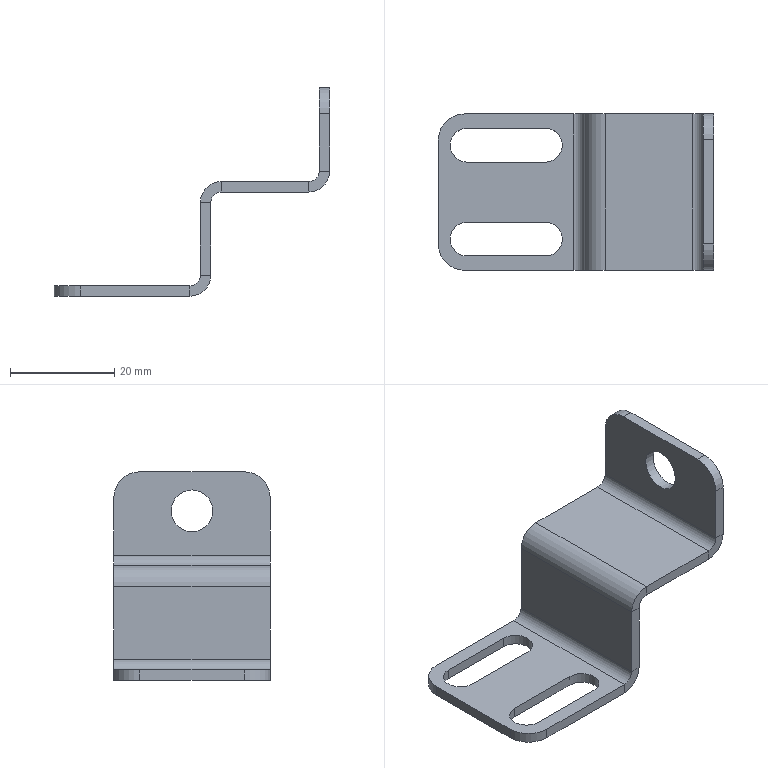Part | STEP file | JBJ-P-1006-10 | 1 solid | 43 faces | box 52.8 x 30 x 40 mm | volume 4550 mm3 | plane 28 | cylinder 15 | commonest cylinder face diameters 6.5 x4 8 x4 10 x4 4 x3
STEP:
#1=CARTESIAN_POINT('',(30.,30.,4.));
#2=VERTEX_POINT('',#1);
#3=CARTESIAN_POINT('',(28.,30.,4.));
#4=VERTEX_POINT('',#3);
#5=CARTESIAN_POINT('',(30.,30.,4.));
#6=DIRECTION('',(-1.,0.,0.));
#7=VECTOR('',#6,1000.);
#8=LINE('',#5,#7);
#9=EDGE_CURVE('',#2,#4,#8,.T.);
#10=ORIENTED_EDGE('',*,*,#9,.F.);
#11=CARTESIAN_POINT('',(26.,30.,0.));
#12=VERTEX_POINT('',#11);
#13=CARTESIAN_POINT('',(26.,30.,4.));
#14=DIRECTION('',(0.,-1.,0.));
#15=DIRECTION('',(0.,0.,1.));
#16=AXIS2_PLACEMENT_3D('',#13,#14,#15);
#17=CIRCLE('',#16,4.);
#18=EDGE_CURVE('',#12,#2,#17,.T.);
#19=ORIENTED_EDGE('',*,*,#18,.F.);
#20=CARTESIAN_POINT('',(26.,30.,2.));
#21=VERTEX_POINT('',#20);
#22=CARTESIAN_POINT('',(26.,30.,2.));
#23=DIRECTION('',(0.,0.,-1.));
#24=VECTOR('',#23,1000.);
#25=LINE('',#22,#24);
#26=EDGE_CURVE('',#21,#12,#25,.T.);
#27=ORIENTED_EDGE('',*,*,#26,.F.);
#28=CARTESIAN_POINT('',(26.,30.,4.));
#29=DIRECTION('',(0.,-1.,0.));
#30=DIRECTION('',(1.,0.,0.));
#31=AXIS2_PLACEMENT_3D('',#28,#29,#30);
#32=CIRCLE('',#31,2.);
#33=EDGE_CURVE('',#21,#4,#32,.T.);
#34=ORIENTED_EDGE('',*,*,#33,.T.);
#35=EDGE_LOOP('',(#10,#19,#27,#34));
#36=FACE_OUTER_BOUND('',#35,.T.);
#37=CARTESIAN_POINT('',(30.,30.,4.));
#38=DIRECTION('',(0.,1.,0.));
#39=DIRECTION('',(0.,0.,1.));
#40=AXIS2_PLACEMENT_3D('',#37,#38,#39);
#41=PLANE('',#40);
#42=ADVANCED_FACE('',(#36),#41,.T.);
#43=CARTESIAN_POINT('',(30.,30.,18.));
#44=VERTEX_POINT('',#43);
#45=CARTESIAN_POINT('',(30.,30.,0.));
#46=DIRECTION('',(0.,0.,1.));
#47=VECTOR('',#46,1000.);
#48=LINE('',#45,#47);
#49=EDGE_CURVE('',#2,#44,#48,.T.);
#50=ORIENTED_EDGE('',*,*,#49,.F.);
#51=ORIENTED_EDGE('',*,*,#9,.T.);
#52=CARTESIAN_POINT('',(28.,30.,18.));
#53=VERTEX_POINT('',#52);
#54=CARTESIAN_POINT('',(28.,30.,0.));
#55=DIRECTION('',(0.,0.,1.));
#56=VECTOR('',#55,1000.);
#57=LINE('',#54,#56);
#58=EDGE_CURVE('',#4,#53,#57,.T.);
#59=ORIENTED_EDGE('',*,*,#58,.T.);
#60=CARTESIAN_POINT('',(28.,30.,18.));
#61=DIRECTION('',(1.,0.,0.));
#62=VECTOR('',#61,1000.);
#63=LINE('',#60,#62);
#64=EDGE_CURVE('',#53,#44,#63,.T.);
#65=ORIENTED_EDGE('',*,*,#64,.T.);
#66=EDGE_LOOP('',(#50,#51,#59,#65));
#67=FACE_OUTER_BOUND('',#66,.T.);
#68=CARTESIAN_POINT('',(26.,30.,2.));
#69=DIRECTION('',(0.,1.,0.));
#70=DIRECTION('',(0.,0.,1.));
#71=AXIS2_PLACEMENT_3D('',#68,#69,#70);
#72=PLANE('',#71);
#73=ADVANCED_FACE('',(#67),#72,.T.);
#74=CARTESIAN_POINT('',(26.,0.,0.));
#75=VERTEX_POINT('',#74);
#76=CARTESIAN_POINT('',(26.,0.,2.));
#77=VERTEX_POINT('',#76);
#78=CARTESIAN_POINT('',(26.,0.,0.));
#79=DIRECTION('',(0.,0.,1.));
#80=VECTOR('',#79,1000.);
#81=LINE('',#78,#80);
#82=EDGE_CURVE('',#75,#77,#81,.T.);
#83=ORIENTED_EDGE('',*,*,#82,.F.);
#84=CARTESIAN_POINT('',(30.,0.,4.));
#85=VERTEX_POINT('',#84);
#86=CARTESIAN_POINT('',(26.,0.,4.));
#87=DIRECTION('',(0.,-1.,0.));
#88=DIRECTION('',(0.,0.,1.));
#89=AXIS2_PLACEMENT_3D('',#86,#87,#88);
#90=CIRCLE('',#89,4.);
#91=EDGE_CURVE('',#75,#85,#90,.T.);
#92=ORIENTED_EDGE('',*,*,#91,.T.);
#93=CARTESIAN_POINT('',(28.,0.,4.));
#94=VERTEX_POINT('',#93);
#95=CARTESIAN_POINT('',(28.,0.,4.));
#96=DIRECTION('',(1.,0.,0.));
#97=VECTOR('',#96,1000.);
#98=LINE('',#95,#97);
#99=EDGE_CURVE('',#94,#85,#98,.T.);
#100=ORIENTED_EDGE('',*,*,#99,.F.);
#101=CARTESIAN_POINT('',(26.,0.,4.));
#102=DIRECTION('',(0.,-1.,0.));
#103=DIRECTION('',(1.,0.,0.));
#104=AXIS2_PLACEMENT_3D('',#101,#102,#103);
#105=CIRCLE('',#104,2.);
#106=EDGE_CURVE('',#77,#94,#105,.T.);
#107=ORIENTED_EDGE('',*,*,#106,.F.);
#108=EDGE_LOOP('',(#83,#92,#100,#107));
#109=FACE_OUTER_BOUND('',#108,.T.);
#110=CARTESIAN_POINT('',(26.,0.,0.));
#111=DIRECTION('',(0.,-1.,0.));
#112=DIRECTION('',(0.,0.,-1.));
#113=AXIS2_PLACEMENT_3D('',#110,#111,#112);
#114=PLANE('',#113);
#115=ADVANCED_FACE('',(#109),#114,.T.);
#116=CARTESIAN_POINT('',(5.,0.,2.));
#117=VERTEX_POINT('',#116);
#118=CARTESIAN_POINT('',(0.,0.,2.));
#119=DIRECTION('',(1.,0.,0.));
#120=VECTOR('',#119,1000.);
#121=LINE('',#118,#120);
#122=EDGE_CURVE('',#117,#77,#121,.T.);
#123=ORIENTED_EDGE('',*,*,#122,.F.);
#124=CARTESIAN_POINT('',(5.,0.,0.));
#125=VERTEX_POINT('',#124);
#126=CARTESIAN_POINT('',(5.,0.,4.));
#127=DIRECTION('',(0.,0.,-1.));
#128=VECTOR('',#127,1000.);
#129=LINE('',#126,#128);
#130=EDGE_CURVE('',#117,#125,#129,.T.);
#131=ORIENTED_EDGE('',*,*,#130,.T.);
#132=CARTESIAN_POINT('',(0.,0.,0.));
#133=DIRECTION('',(1.,0.,0.));
#134=VECTOR('',#133,1000.);
#135=LINE('',#132,#134);
#136=EDGE_CURVE('',#125,#75,#135,.T.);
#137=ORIENTED_EDGE('',*,*,#136,.T.);
#138=ORIENTED_EDGE('',*,*,#82,.T.);
#139=EDGE_LOOP('',(#123,#131,#137,#138));
#140=FACE_OUTER_BOUND('',#139,.T.);
#141=CARTESIAN_POINT('',(28.,0.,4.));
#142=DIRECTION('',(0.,-1.,0.));
#143=DIRECTION('',(0.,0.,-1.));
#144=AXIS2_PLACEMENT_3D('',#141,#142,#143);
#145=PLANE('',#144);
#146=ADVANCED_FACE('',(#140),#145,.T.);
#147=CARTESIAN_POINT('',(32.,30.,20.));
#148=VERTEX_POINT('',#147);
#149=CARTESIAN_POINT('',(32.,30.,22.));
#150=VERTEX_POINT('',#149);
#151=CARTESIAN_POINT('',(32.,30.,20.));
#152=DIRECTION('',(0.,0.,1.));
#153=VECTOR('',#152,1000.);
#154=LINE('',#151,#153);
#155=EDGE_CURVE('',#148,#150,#154,.T.);
#156=ORIENTED_EDGE('',*,*,#155,.F.);
#157=CARTESIAN_POINT('',(32.,30.,18.));
#158=DIRECTION('',(0.,1.,0.));
#159=DIRECTION('',(0.,0.,-1.));
#160=AXIS2_PLACEMENT_3D('',#157,#158,#159);
#161=CIRCLE('',#160,2.);
#162=EDGE_CURVE('',#44,#148,#161,.T.);
#163=ORIENTED_EDGE('',*,*,#162,.F.);
#164=ORIENTED_EDGE('',*,*,#64,.F.);
#165=CARTESIAN_POINT('',(32.,30.,18.));
#166=DIRECTION('',(0.,1.,0.));
#167=DIRECTION('',(1.,0.,0.));
#168=AXIS2_PLACEMENT_3D('',#165,#166,#167);
#169=CIRCLE('',#168,4.);
#170=EDGE_CURVE('',#53,#150,#169,.T.);
#171=ORIENTED_EDGE('',*,*,#170,.T.);
#172=EDGE_LOOP('',(#156,#163,#164,#171));
#173=FACE_OUTER_BOUND('',#172,.T.);
#174=CARTESIAN_POINT('',(32.,30.,20.));
#175=DIRECTION('',(0.,1.,0.));
#176=DIRECTION('',(0.,0.,1.));
#177=AXIS2_PLACEMENT_3D('',#174,#175,#176);
#178=PLANE('',#177);
#179=ADVANCED_FACE('',(#173),#178,.T.);
#180=CARTESIAN_POINT('',(48.8,30.,20.));
#181=VERTEX_POINT('',#180);
#182=CARTESIAN_POINT('',(30.,30.,20.));
#183=DIRECTION('',(1.,0.,0.));
#184=VECTOR('',#183,1000.);
#185=LINE('',#182,#184);
#186=EDGE_CURVE('',#148,#181,#185,.T.);
#187=ORIENTED_EDGE('',*,*,#186,.F.);
#188=ORIENTED_EDGE('',*,*,#155,.T.);
#189=CARTESIAN_POINT('',(48.8,30.,22.));
#190=VERTEX_POINT('',#189);
#191=CARTESIAN_POINT('',(30.,30.,22.));
#192=DIRECTION('',(1.,0.,0.));
#193=VECTOR('',#192,1000.);
#194=LINE('',#191,#193);
#195=EDGE_CURVE('',#150,#190,#194,.T.);
#196=ORIENTED_EDGE('',*,*,#195,.T.);
#197=CARTESIAN_POINT('',(48.8,30.,22.));
#198=DIRECTION('',(0.,0.,-1.));
#199=VECTOR('',#198,1000.);
#200=LINE('',#197,#199);
#201=EDGE_CURVE('',#190,#181,#200,.T.);
#202=ORIENTED_EDGE('',*,*,#201,.T.);
#203=EDGE_LOOP('',(#187,#188,#196,#202));
#204=FACE_OUTER_BOUND('',#203,.T.);
#205=CARTESIAN_POINT('',(28.,30.,18.));
#206=DIRECTION('',(0.,1.,0.));
#207=DIRECTION('',(0.,0.,1.));
#208=AXIS2_PLACEMENT_3D('',#205,#206,#207);
#209=PLANE('',#208);
#210=ADVANCED_FACE('',(#204),#209,.T.);
#211=CARTESIAN_POINT('',(30.,0.,18.));
#212=VERTEX_POINT('',#211);
#213=CARTESIAN_POINT('',(28.,0.,18.));
#214=VERTEX_POINT('',#213);
#215=CARTESIAN_POINT('',(30.,0.,18.));
#216=DIRECTION('',(-1.,0.,0.));
#217=VECTOR('',#216,1000.);
#218=LINE('',#215,#217);
#219=EDGE_CURVE('',#212,#214,#218,.T.);
#220=ORIENTED_EDGE('',*,*,#219,.F.);
#221=CARTESIAN_POINT('',(32.,0.,20.));
#222=VERTEX_POINT('',#221);
#223=CARTESIAN_POINT('',(32.,0.,18.));
#224=DIRECTION('',(0.,1.,0.));
#225=DIRECTION('',(0.,0.,-1.));
#226=AXIS2_PLACEMENT_3D('',#223,#224,#225);
#227=CIRCLE('',#226,2.);
#228=EDGE_CURVE('',#212,#222,#227,.T.);
#229=ORIENTED_EDGE('',*,*,#228,.T.);
#230=CARTESIAN_POINT('',(32.,0.,22.));
#231=VERTEX_POINT('',#230);
#232=CARTESIAN_POINT('',(32.,0.,22.));
#233=DIRECTION('',(0.,0.,-1.));
#234=VECTOR('',#233,1000.);
#235=LINE('',#232,#234);
#236=EDGE_CURVE('',#231,#222,#235,.T.);
#237=ORIENTED_EDGE('',*,*,#236,.F.);
#238=CARTESIAN_POINT('',(32.,0.,18.));
#239=DIRECTION('',(0.,1.,0.));
#240=DIRECTION('',(1.,0.,0.));
#241=AXIS2_PLACEMENT_3D('',#238,#239,#240);
#242=CIRCLE('',#241,4.);
#243=EDGE_CURVE('',#214,#231,#242,.T.);
#244=ORIENTED_EDGE('',*,*,#243,.F.);
#245=EDGE_LOOP('',(#220,#229,#237,#244));
#246=FACE_OUTER_BOUND('',#245,.T.);
#247=CARTESIAN_POINT('',(30.,0.,18.));
#248=DIRECTION('',(0.,-1.,0.));
#249=DIRECTION('',(0.,0.,-1.));
#250=AXIS2_PLACEMENT_3D('',#247,#248,#249);
#251=PLANE('',#250);
#252=ADVANCED_FACE('',(#246),#251,.T.);
#253=CARTESIAN_POINT('',(30.,0.,0.));
#254=DIRECTION('',(0.,0.,1.));
#255=VECTOR('',#254,1000.);
#256=LINE('',#253,#255);
#257=EDGE_CURVE('',#85,#212,#256,.T.);
#258=ORIENTED_EDGE('',*,*,#257,.T.);
#259=ORIENTED_EDGE('',*,*,#219,.T.);
#260=CARTESIAN_POINT('',(28.,0.,0.));
#261=DIRECTION('',(0.,0.,1.));
#262=VECTOR('',#261,1000.);
#263=LINE('',#260,#262);
#264=EDGE_CURVE('',#94,#214,#263,.T.);
#265=ORIENTED_EDGE('',*,*,#264,.F.);
#266=ORIENTED_EDGE('',*,*,#99,.T.);
#267=EDGE_LOOP('',(#258,#259,#265,#266));
#268=FACE_OUTER_BOUND('',#267,.T.);
#269=CARTESIAN_POINT('',(32.,0.,22.));
#270=DIRECTION('',(0.,-1.,0.));
#271=DIRECTION('',(0.,0.,-1.));
#272=AXIS2_PLACEMENT_3D('',#269,#270,#271);
#273=PLANE('',#272);
#274=ADVANCED_FACE('',(#268),#273,.T.);
#275=CARTESIAN_POINT('',(52.8,30.,24.));
#276=VERTEX_POINT('',#275);
#277=CARTESIAN_POINT('',(50.8,30.,24.));
#278=VERTEX_POINT('',#277);
#279=CARTESIAN_POINT('',(52.8,30.,24.));
#280=DIRECTION('',(-1.,0.,0.));
#281=VECTOR('',#280,1000.);
#282=LINE('',#279,#281);
#283=EDGE_CURVE('',#276,#278,#282,.T.);
#284=ORIENTED_EDGE('',*,*,#283,.F.);
#285=CARTESIAN_POINT('',(48.8,30.,24.));
#286=DIRECTION('',(0.,-1.,0.));
#287=DIRECTION('',(0.,0.,1.));
#288=AXIS2_PLACEMENT_3D('',#285,#286,#287);
#289=CIRCLE('',#288,4.);
#290=EDGE_CURVE('',#181,#276,#289,.T.);
#291=ORIENTED_EDGE('',*,*,#290,.F.);
#292=ORIENTED_EDGE('',*,*,#201,.F.);
#293=CARTESIAN_POINT('',(48.8,30.,24.));
#294=DIRECTION('',(0.,-1.,0.));
#295=DIRECTION('',(1.,0.,0.));
#296=AXIS2_PLACEMENT_3D('',#293,#294,#295);
#297=CIRCLE('',#296,2.);
#298=EDGE_CURVE('',#190,#278,#297,.T.);
#299=ORIENTED_EDGE('',*,*,#298,.T.);
#300=EDGE_LOOP('',(#284,#291,#292,#299));
#301=FACE_OUTER_BOUND('',#300,.T.);
#302=CARTESIAN_POINT('',(52.8,30.,24.));
#303=DIRECTION('',(0.,1.,0.));
#304=DIRECTION('',(0.,0.,1.));
#305=AXIS2_PLACEMENT_3D('',#302,#303,#304);
#306=PLANE('',#305);
#307=ADVANCED_FACE('',(#301),#306,.T.);
#308=CARTESIAN_POINT('',(50.8,30.,35.));
#309=VERTEX_POINT('',#308);
#310=CARTESIAN_POINT('',(50.8,30.,20.));
#311=DIRECTION('',(0.,0.,1.));
#312=VECTOR('',#311,1000.);
#313=LINE('',#310,#312);
#314=EDGE_CURVE('',#278,#309,#313,.T.);
#315=ORIENTED_EDGE('',*,*,#314,.T.);
#316=CARTESIAN_POINT('',(52.8,30.,35.));
#317=VERTEX_POINT('',#316);
#318=CARTESIAN_POINT('',(48.8,30.,35.));
#319=DIRECTION('',(1.,0.,0.));
#320=VECTOR('',#319,1000.);
#321=LINE('',#318,#320);
#322=EDGE_CURVE('',#309,#317,#321,.T.);
#323=ORIENTED_EDGE('',*,*,#322,.T.);
#324=CARTESIAN_POINT('',(52.8,30.,20.));
#325=DIRECTION('',(0.,0.,1.));
#326=VECTOR('',#325,1000.);
#327=LINE('',#324,#326);
#328=EDGE_CURVE('',#276,#317,#327,.T.);
#329=ORIENTED_EDGE('',*,*,#328,.F.);
#330=ORIENTED_EDGE('',*,*,#283,.T.);
#331=EDGE_LOOP('',(#315,#323,#329,#330));
#332=FACE_OUTER_BOUND('',#331,.T.);
#333=CARTESIAN_POINT('',(48.8,30.,22.));
#334=DIRECTION('',(0.,1.,0.));
#335=DIRECTION('',(0.,0.,1.));
#336=AXIS2_PLACEMENT_3D('',#333,#334,#335);
#337=PLANE('',#336);
#338=ADVANCED_FACE('',(#332),#337,.T.);
#339=CARTESIAN_POINT('',(48.8,0.,20.));
#340=VERTEX_POINT('',#339);
#341=CARTESIAN_POINT('',(48.8,0.,22.));
#342=VERTEX_POINT('',#341);
#343=CARTESIAN_POINT('',(48.8,0.,20.));
#344=DIRECTION('',(0.,0.,1.));
#345=VECTOR('',#344,1000.);
#346=LINE('',#343,#345);
#347=EDGE_CURVE('',#340,#342,#346,.T.);
#348=ORIENTED_EDGE('',*,*,#347,.F.);
#349=CARTESIAN_POINT('',(52.8,0.,24.));
#350=VERTEX_POINT('',#349);
#351=CARTESIAN_POINT('',(48.8,0.,24.));
#352=DIRECTION('',(0.,-1.,0.));
#353=DIRECTION('',(0.,0.,1.));
#354=AXIS2_PLACEMENT_3D('',#351,#352,#353);
#355=CIRCLE('',#354,4.);
#356=EDGE_CURVE('',#340,#350,#355,.T.);
#357=ORIENTED_EDGE('',*,*,#356,.T.);
#358=CARTESIAN_POINT('',(50.8,0.,24.));
#359=VERTEX_POINT('',#358);
#360=CARTESIAN_POINT('',(50.8,0.,24.));
#361=DIRECTION('',(1.,0.,0.));
#362=VECTOR('',#361,1000.);
#363=LINE('',#360,#362);
#364=EDGE_CURVE('',#359,#350,#363,.T.);
#365=ORIENTED_EDGE('',*,*,#364,.F.);
#366=CARTESIAN_POINT('',(48.8,0.,24.));
#367=DIRECTION('',(0.,-1.,0.));
#368=DIRECTION('',(1.,0.,0.));
#369=AXIS2_PLACEMENT_3D('',#366,#367,#368);
#370=CIRCLE('',#369,2.);
#371=EDGE_CURVE('',#342,#359,#370,.T.);
#372=ORIENTED_EDGE('',*,*,#371,.F.);
#373=EDGE_LOOP('',(#348,#357,#365,#372));
#374=FACE_OUTER_BOUND('',#373,.T.);
#375=CARTESIAN_POINT('',(48.8,0.,20.));
#376=DIRECTION('',(0.,-1.,0.));
#377=DIRECTION('',(0.,0.,-1.));
#378=AXIS2_PLACEMENT_3D('',#375,#376,#377);
#379=PLANE('',#378);
#380=ADVANCED_FACE('',(#374),#379,.T.);
#381=CARTESIAN_POINT('',(30.,0.,20.));
#382=DIRECTION('',(1.,0.,0.));
#383=VECTOR('',#382,1000.);
#384=LINE('',#381,#383);
#385=EDGE_CURVE('',#222,#340,#384,.T.);
#386=ORIENTED_EDGE('',*,*,#385,.T.);
#387=ORIENTED_EDGE('',*,*,#347,.T.);
#388=CARTESIAN_POINT('',(30.,0.,22.));
#389=DIRECTION('',(1.,0.,0.));
#390=VECTOR('',#389,1000.);
#391=LINE('',#388,#390);
#392=EDGE_CURVE('',#231,#342,#391,.T.);
#393=ORIENTED_EDGE('',*,*,#392,.F.);
#394=ORIENTED_EDGE('',*,*,#236,.T.);
#395=EDGE_LOOP('',(#386,#387,#393,#394));
#396=FACE_OUTER_BOUND('',#395,.T.);
#397=CARTESIAN_POINT('',(50.8,0.,24.));
#398=DIRECTION('',(0.,-1.,0.));
#399=DIRECTION('',(0.,0.,-1.));
#400=AXIS2_PLACEMENT_3D('',#397,#398,#399);
#401=PLANE('',#400);
#402=ADVANCED_FACE('',(#396),#401,.T.);
#403=CARTESIAN_POINT('',(50.8,15.,36.5));
#404=VERTEX_POINT('',#403);
#405=CARTESIAN_POINT('',(50.8,15.,32.5));
#406=DIRECTION('',(-1.,0.,0.));
#407=DIRECTION('',(0.,0.,1.));
#408=AXIS2_PLACEMENT_3D('',#405,#406,#407);
#409=CIRCLE('',#408,4.);
#410=EDGE_CURVE('',#404,#404,#409,.T.);
#411=ORIENTED_EDGE('',*,*,#410,.F.);
#412=EDGE_LOOP('',(#411));
#413=FACE_BOUND('',#412,.T.);
#414=CARTESIAN_POINT('',(50.8,0.,35.));
#415=VERTEX_POINT('',#414);
#416=CARTESIAN_POINT('',(50.8,0.,20.));
#417=DIRECTION('',(0.,0.,1.));
#418=VECTOR('',#417,1000.);
#419=LINE('',#416,#418);
#420=EDGE_CURVE('',#359,#415,#419,.T.);
#421=ORIENTED_EDGE('',*,*,#420,.T.);
#422=CARTESIAN_POINT('',(50.8,5.,40.));
#423=VERTEX_POINT('',#422);
#424=CARTESIAN_POINT('',(50.8,5.,35.));
#425=DIRECTION('',(-1.,0.,0.));
#426=DIRECTION('',(0.,0.,-1.));
#427=AXIS2_PLACEMENT_3D('',#424,#425,#426);
#428=CIRCLE('',#427,5.);
#429=EDGE_CURVE('',#415,#423,#428,.T.);
#430=ORIENTED_EDGE('',*,*,#429,.T.);
#431=CARTESIAN_POINT('',(50.8,25.,40.));
#432=VERTEX_POINT('',#431);
#433=CARTESIAN_POINT('',(50.8,30.,40.));
#434=DIRECTION('',(0.,-1.,0.));
#435=VECTOR('',#434,1000.);
#436=LINE('',#433,#435);
#437=EDGE_CURVE('',#432,#423,#436,.T.);
#438=ORIENTED_EDGE('',*,*,#437,.F.);
#439=CARTESIAN_POINT('',(50.8,25.,35.));
#440=DIRECTION('',(-1.,0.,0.));
#441=DIRECTION('',(0.,0.,-1.));
#442=AXIS2_PLACEMENT_3D('',#439,#440,#441);
#443=CIRCLE('',#442,5.);
#444=EDGE_CURVE('',#432,#309,#443,.T.);
#445=ORIENTED_EDGE('',*,*,#444,.T.);
#446=ORIENTED_EDGE('',*,*,#314,.F.);
#447=CARTESIAN_POINT('',(50.8,30.,24.));
#448=DIRECTION('',(0.,-1.,0.));
#449=VECTOR('',#448,1000.);
#450=LINE('',#447,#449);
#451=EDGE_CURVE('',#278,#359,#450,.T.);
#452=ORIENTED_EDGE('',*,*,#451,.T.);
#453=EDGE_LOOP('',(#421,#430,#438,#445,#446,#452));
#454=FACE_OUTER_BOUND('',#453,.T.);
#455=CARTESIAN_POINT('',(50.8,30.,20.));
#456=DIRECTION('',(1.,0.,0.));
#457=DIRECTION('',(0.,0.,-1.));
#458=AXIS2_PLACEMENT_3D('',#455,#456,#457);
#459=PLANE('',#458);
#460=ADVANCED_FACE('',(#413,#454),#459,.F.);
#461=ORIENTED_EDGE('',*,*,#437,.T.);
#462=CARTESIAN_POINT('',(52.8,5.,40.));
#463=VERTEX_POINT('',#462);
#464=CARTESIAN_POINT('',(52.8,5.,40.));
#465=DIRECTION('',(1.,0.,0.));
#466=VECTOR('',#465,1000.);
#467=LINE('',#464,#466);
#468=EDGE_CURVE('',#423,#463,#467,.T.);
#469=ORIENTED_EDGE('',*,*,#468,.T.);
#470=CARTESIAN_POINT('',(52.8,25.,40.));
#471=VERTEX_POINT('',#470);
#472=CARTESIAN_POINT('',(52.8,30.,40.));
#473=DIRECTION('',(0.,-1.,0.));
#474=VECTOR('',#473,1000.);
#475=LINE('',#472,#474);
#476=EDGE_CURVE('',#471,#463,#475,.T.);
#477=ORIENTED_EDGE('',*,*,#476,.F.);
#478=CARTESIAN_POINT('',(52.8,25.,40.));
#479=DIRECTION('',(-1.,0.,0.));
#480=VECTOR('',#479,1000.);
#481=LINE('',#478,#480);
#482=EDGE_CURVE('',#471,#432,#481,.T.);
#483=ORIENTED_EDGE('',*,*,#482,.T.);
#484=EDGE_LOOP('',(#461,#469,#477,#483));
#485=FACE_OUTER_BOUND('',#484,.T.);
#486=CARTESIAN_POINT('',(52.8,30.,40.));
#487=DIRECTION('',(0.,0.,1.));
#488=DIRECTION('',(1.,0.,0.));
#489=AXIS2_PLACEMENT_3D('',#486,#487,#488);
#490=PLANE('',#489);
#491=ADVANCED_FACE('',(#485),#490,.T.);
#492=CARTESIAN_POINT('',(52.8,15.,28.5));
#493=VERTEX_POINT('',#492);
#494=CARTESIAN_POINT('',(52.8,15.,32.5));
#495=DIRECTION('',(1.,0.,0.));
#496=DIRECTION('',(0.,0.,-1.));
#497=AXIS2_PLACEMENT_3D('',#494,#495,#496);
#498=CIRCLE('',#497,4.);
#499=EDGE_CURVE('',#493,#493,#498,.T.);
#500=ORIENTED_EDGE('',*,*,#499,.F.);
#501=EDGE_LOOP('',(#500));
#502=FACE_BOUND('',#501,.T.);
#503=ORIENTED_EDGE('',*,*,#476,.T.);
#504=CARTESIAN_POINT('',(52.8,0.,35.));
#505=VERTEX_POINT('',#504);
#506=CARTESIAN_POINT('',(52.8,5.,35.));
#507=DIRECTION('',(1.,0.,0.));
#508=DIRECTION('',(0.,0.,-1.));
#509=AXIS2_PLACEMENT_3D('',#506,#507,#508);
#510=CIRCLE('',#509,5.);
#511=EDGE_CURVE('',#463,#505,#510,.T.);
#512=ORIENTED_EDGE('',*,*,#511,.T.);
#513=CARTESIAN_POINT('',(52.8,0.,20.));
#514=DIRECTION('',(0.,0.,1.));
#515=VECTOR('',#514,1000.);
#516=LINE('',#513,#515);
#517=EDGE_CURVE('',#350,#505,#516,.T.);
#518=ORIENTED_EDGE('',*,*,#517,.F.);
#519=CARTESIAN_POINT('',(52.8,30.,24.));
#520=DIRECTION('',(0.,-1.,0.));
#521=VECTOR('',#520,1000.);
#522=LINE('',#519,#521);
#523=EDGE_CURVE('',#276,#350,#522,.T.);
#524=ORIENTED_EDGE('',*,*,#523,.F.);
#525=ORIENTED_EDGE('',*,*,#328,.T.);
#526=CARTESIAN_POINT('',(52.8,25.,35.));
#527=DIRECTION('',(1.,0.,0.));
#528=DIRECTION('',(0.,0.,-1.));
#529=AXIS2_PLACEMENT_3D('',#526,#527,#528);
#530=CIRCLE('',#529,5.);
#531=EDGE_CURVE('',#317,#471,#530,.T.);
#532=ORIENTED_EDGE('',*,*,#531,.T.);
#533=EDGE_LOOP('',(#503,#512,#518,#524,#525,#532));
#534=FACE_OUTER_BOUND('',#533,.T.);
#535=CARTESIAN_POINT('',(52.8,30.,20.));
#536=DIRECTION('',(1.,0.,0.));
#537=DIRECTION('',(0.,0.,-1.));
#538=AXIS2_PLACEMENT_3D('',#535,#536,#537);
#539=PLANE('',#538);
#540=ADVANCED_FACE('',(#502,#534),#539,.T.);
#541=ORIENTED_EDGE('',*,*,#356,.F.);
#542=CARTESIAN_POINT('',(48.8,30.,20.));
#543=DIRECTION('',(0.,-1.,0.));
#544=VECTOR('',#543,1000.);
#545=LINE('',#542,#544);
#546=EDGE_CURVE('',#181,#340,#545,.T.);
#547=ORIENTED_EDGE('',*,*,#546,.F.);
#548=ORIENTED_EDGE('',*,*,#290,.T.);
#549=ORIENTED_EDGE('',*,*,#523,.T.);
#550=EDGE_LOOP('',(#541,#547,#548,#549));
#551=FACE_OUTER_BOUND('',#550,.T.);
#552=CARTESIAN_POINT('',(48.8,30.,24.));
#553=DIRECTION('',(0.,-1.,0.));
#554=DIRECTION('',(0.,0.,-1.));
#555=AXIS2_PLACEMENT_3D('',#552,#553,#554);
#556=CYLINDRICAL_SURFACE('',#555,4.);
#557=ADVANCED_FACE('',(#551),#556,.T.);
#558=ORIENTED_EDGE('',*,*,#385,.F.);
#559=CARTESIAN_POINT('',(32.,30.,20.));
#560=DIRECTION('',(0.,-1.,0.));
#561=VECTOR('',#560,1000.);
#562=LINE('',#559,#561);
#563=EDGE_CURVE('',#148,#222,#562,.T.);
#564=ORIENTED_EDGE('',*,*,#563,.F.);
#565=ORIENTED_EDGE('',*,*,#186,.T.);
#566=ORIENTED_EDGE('',*,*,#546,.T.);
#567=EDGE_LOOP('',(#558,#564,#565,#566));
#568=FACE_OUTER_BOUND('',#567,.T.);
#569=CARTESIAN_POINT('',(30.,30.,20.));
#570=DIRECTION('',(0.,0.,-1.));
#571=DIRECTION('',(-1.,0.,0.));
#572=AXIS2_PLACEMENT_3D('',#569,#570,#571);
#573=PLANE('',#572);
#574=ADVANCED_FACE('',(#568),#573,.T.);
#575=ORIENTED_EDGE('',*,*,#228,.F.);
#576=CARTESIAN_POINT('',(30.,30.,18.));
#577=DIRECTION('',(0.,-1.,0.));
#578=VECTOR('',#577,1000.);
#579=LINE('',#576,#578);
#580=EDGE_CURVE('',#44,#212,#579,.T.);
#581=ORIENTED_EDGE('',*,*,#580,.F.);
#582=ORIENTED_EDGE('',*,*,#162,.T.);
#583=ORIENTED_EDGE('',*,*,#563,.T.);
#584=EDGE_LOOP('',(#575,#581,#582,#583));
#585=FACE_OUTER_BOUND('',#584,.T.);
#586=CARTESIAN_POINT('',(32.,30.,18.));
#587=DIRECTION('',(0.,-1.,0.));
#588=DIRECTION('',(0.,0.,-1.));
#589=AXIS2_PLACEMENT_3D('',#586,#587,#588);
#590=CYLINDRICAL_SURFACE('',#589,2.);
#591=ADVANCED_FACE('',(#585),#590,.F.);
#592=ORIENTED_EDGE('',*,*,#257,.F.);
#593=CARTESIAN_POINT('',(30.,30.,4.));
#594=DIRECTION('',(0.,-1.,0.));
#595=VECTOR('',#594,1000.);
#596=LINE('',#593,#595);
#597=EDGE_CURVE('',#2,#85,#596,.T.);
#598=ORIENTED_EDGE('',*,*,#597,.F.);
#599=ORIENTED_EDGE('',*,*,#49,.T.);
#600=ORIENTED_EDGE('',*,*,#580,.T.);
#601=EDGE_LOOP('',(#592,#598,#599,#600));
#602=FACE_OUTER_BOUND('',#601,.T.);
#603=CARTESIAN_POINT('',(30.,30.,0.));
#604=DIRECTION('',(1.,0.,0.));
#605=DIRECTION('',(0.,0.,-1.));
#606=AXIS2_PLACEMENT_3D('',#603,#604,#605);
#607=PLANE('',#606);
#608=ADVANCED_FACE('',(#602),#607,.T.);
#609=ORIENTED_EDGE('',*,*,#91,.F.);
#610=CARTESIAN_POINT('',(26.,30.,0.));
#611=DIRECTION('',(0.,-1.,0.));
#612=VECTOR('',#611,1000.);
#613=LINE('',#610,#612);
#614=EDGE_CURVE('',#12,#75,#613,.T.);
#615=ORIENTED_EDGE('',*,*,#614,.F.);
#616=ORIENTED_EDGE('',*,*,#18,.T.);
#617=ORIENTED_EDGE('',*,*,#597,.T.);
#618=EDGE_LOOP('',(#609,#615,#616,#617));
#619=FACE_OUTER_BOUND('',#618,.T.);
#620=CARTESIAN_POINT('',(26.,30.,4.));
#621=DIRECTION('',(0.,-1.,0.));
#622=DIRECTION('',(0.,0.,-1.));
#623=AXIS2_PLACEMENT_3D('',#620,#621,#622);
#624=CYLINDRICAL_SURFACE('',#623,4.);
#625=ADVANCED_FACE('',(#619),#624,.T.);
#626=CARTESIAN_POINT('',(20.5,27.25,0.));
#627=VERTEX_POINT('',#626);
#628=CARTESIAN_POINT('',(20.5,20.75,0.));
#629=VERTEX_POINT('',#628);
#630=CARTESIAN_POINT('',(20.5,24.,0.));
#631=DIRECTION('',(0.,0.,-1.));
#632=DIRECTION('',(-1.,0.,0.));
#633=AXIS2_PLACEMENT_3D('',#630,#631,#632);
#634=CIRCLE('',#633,3.25);
#635=EDGE_CURVE('',#627,#629,#634,.T.);
#636=ORIENTED_EDGE('',*,*,#635,.F.);
#637=CARTESIAN_POINT('',(5.5,27.25,0.));
#638=VERTEX_POINT('',#637);
#639=CARTESIAN_POINT('',(20.5,27.25,0.));
#640=DIRECTION('',(1.,0.,0.));
#641=VECTOR('',#640,1000.);
#642=LINE('',#639,#641);
#643=EDGE_CURVE('',#638,#627,#642,.T.);
#644=ORIENTED_EDGE('',*,*,#643,.F.);
#645=CARTESIAN_POINT('',(5.5,20.75,0.));
#646=VERTEX_POINT('',#645);
#647=CARTESIAN_POINT('',(5.5,24.,0.));
#648=DIRECTION('',(0.,0.,-1.));
#649=DIRECTION('',(-1.,0.,0.));
#650=AXIS2_PLACEMENT_3D('',#647,#648,#649);
#651=CIRCLE('',#650,3.25);
#652=EDGE_CURVE('',#646,#638,#651,.T.);
#653=ORIENTED_EDGE('',*,*,#652,.F.);
#654=CARTESIAN_POINT('',(20.5,20.75,0.));
#655=DIRECTION('',(-1.,0.,0.));
#656=VECTOR('',#655,1000.);
#657=LINE('',#654,#656);
#658=EDGE_CURVE('',#629,#646,#657,.T.);
#659=ORIENTED_EDGE('',*,*,#658,.F.);
#660=EDGE_LOOP('',(#636,#644,#653,#659));
#661=FACE_BOUND('',#660,.T.);
#662=CARTESIAN_POINT('',(20.5,9.25,0.));
#663=VERTEX_POINT('',#662);
#664=CARTESIAN_POINT('',(20.5,2.75,0.));
#665=VERTEX_POINT('',#664);
#666=CARTESIAN_POINT('',(20.5,6.,0.));
#667=DIRECTION('',(0.,0.,-1.));
#668=DIRECTION('',(1.,0.,0.));
#669=AXIS2_PLACEMENT_3D('',#666,#667,#668);
#670=CIRCLE('',#669,3.25);
#671=EDGE_CURVE('',#663,#665,#670,.T.);
#672=ORIENTED_EDGE('',*,*,#671,.F.);
#673=CARTESIAN_POINT('',(5.5,9.25,0.));
#674=VERTEX_POINT('',#673);
#675=CARTESIAN_POINT('',(20.5,9.25,0.));
#676=DIRECTION('',(1.,0.,0.));
#677=VECTOR('',#676,1000.);
#678=LINE('',#675,#677);
#679=EDGE_CURVE('',#674,#663,#678,.T.);
#680=ORIENTED_EDGE('',*,*,#679,.F.);
#681=CARTESIAN_POINT('',(5.5,2.75,0.));
#682=VERTEX_POINT('',#681);
#683=CARTESIAN_POINT('',(5.5,6.,0.));
#684=DIRECTION('',(0.,0.,-1.));
#685=DIRECTION('',(1.,0.,0.));
#686=AXIS2_PLACEMENT_3D('',#683,#684,#685);
#687=CIRCLE('',#686,3.25);
#688=EDGE_CURVE('',#682,#674,#687,.T.);
#689=ORIENTED_EDGE('',*,*,#688,.F.);
#690=CARTESIAN_POINT('',(20.5,2.75,0.));
#691=DIRECTION('',(-1.,0.,0.));
#692=VECTOR('',#691,1000.);
#693=LINE('',#690,#692);
#694=EDGE_CURVE('',#665,#682,#693,.T.);
#695=ORIENTED_EDGE('',*,*,#694,.F.);
#696=EDGE_LOOP('',(#672,#680,#689,#695));
#697=FACE_BOUND('',#696,.T.);
#698=CARTESIAN_POINT('',(0.,25.,0.));
#699=VERTEX_POINT('',#698);
#700=CARTESIAN_POINT('',(0.,5.,0.));
#701=VERTEX_POINT('',#700);
#702=CARTESIAN_POINT('',(0.,30.,0.));
#703=DIRECTION('',(0.,-1.,0.));
#704=VECTOR('',#703,1000.);
#705=LINE('',#702,#704);
#706=EDGE_CURVE('',#699,#701,#705,.T.);
#707=ORIENTED_EDGE('',*,*,#706,.F.);
#708=CARTESIAN_POINT('',(5.,30.,0.));
#709=VERTEX_POINT('',#708);
#710=CARTESIAN_POINT('',(5.,25.,0.));
#711=DIRECTION('',(0.,0.,-1.));
#712=DIRECTION('',(-1.,0.,0.));
#713=AXIS2_PLACEMENT_3D('',#710,#711,#712);
#714=CIRCLE('',#713,5.);
#715=EDGE_CURVE('',#699,#709,#714,.T.);
#716=ORIENTED_EDGE('',*,*,#715,.T.);
#717=CARTESIAN_POINT('',(0.,30.,0.));
#718=DIRECTION('',(1.,0.,0.));
#719=VECTOR('',#718,1000.);
#720=LINE('',#717,#719);
#721=EDGE_CURVE('',#709,#12,#720,.T.);
#722=ORIENTED_EDGE('',*,*,#721,.T.);
#723=ORIENTED_EDGE('',*,*,#614,.T.);
#724=ORIENTED_EDGE('',*,*,#136,.F.);
#725=CARTESIAN_POINT('',(5.,5.,0.));
#726=DIRECTION('',(0.,0.,-1.));
#727=DIRECTION('',(-1.,0.,0.));
#728=AXIS2_PLACEMENT_3D('',#725,#726,#727);
#729=CIRCLE('',#728,5.);
#730=EDGE_CURVE('',#125,#701,#729,.T.);
#731=ORIENTED_EDGE('',*,*,#730,.T.);
#732=EDGE_LOOP('',(#707,#716,#722,#723,#724,#731));
#733=FACE_OUTER_BOUND('',#732,.T.);
#734=CARTESIAN_POINT('',(0.,30.,0.));
#735=DIRECTION('',(0.,0.,-1.));
#736=DIRECTION('',(-1.,0.,0.));
#737=AXIS2_PLACEMENT_3D('',#734,#735,#736);
#738=PLANE('',#737);
#739=ADVANCED_FACE('',(#661,#697,#733),#738,.T.);
#740=CARTESIAN_POINT('',(0.,25.,2.));
#741=VERTEX_POINT('',#740);
#742=CARTESIAN_POINT('',(0.,5.,2.));
#743=VERTEX_POINT('',#742);
#744=CARTESIAN_POINT('',(0.,30.,2.));
#745=DIRECTION('',(0.,-1.,0.));
#746=VECTOR('',#745,1000.);
#747=LINE('',#744,#746);
#748=EDGE_CURVE('',#741,#743,#747,.T.);
#749=ORIENTED_EDGE('',*,*,#748,.F.);
#750=CARTESIAN_POINT('',(0.,25.,2.));
#751=DIRECTION('',(0.,0.,-1.));
#752=VECTOR('',#751,1000.);
#753=LINE('',#750,#752);
#754=EDGE_CURVE('',#741,#699,#753,.T.);
#755=ORIENTED_EDGE('',*,*,#754,.T.);
#756=ORIENTED_EDGE('',*,*,#706,.T.);
#757=CARTESIAN_POINT('',(0.,5.,2.));
#758=DIRECTION('',(0.,0.,1.));
#759=VECTOR('',#758,1000.);
#760=LINE('',#757,#759);
#761=EDGE_CURVE('',#701,#743,#760,.T.);
#762=ORIENTED_EDGE('',*,*,#761,.T.);
#763=EDGE_LOOP('',(#749,#755,#756,#762));
#764=FACE_OUTER_BOUND('',#763,.T.);
#765=CARTESIAN_POINT('',(0.,30.,2.));
#766=DIRECTION('',(-1.,0.,0.));
#767=DIRECTION('',(0.,0.,1.));
#768=AXIS2_PLACEMENT_3D('',#765,#766,#767);
#769=PLANE('',#768);
#770=ADVANCED_FACE('',(#764),#769,.T.);
#771=CARTESIAN_POINT('',(5.5,27.25,2.));
#772=VERTEX_POINT('',#771);
#773=CARTESIAN_POINT('',(20.5,27.25,2.));
#774=VERTEX_POINT('',#773);
#775=CARTESIAN_POINT('',(0.,27.25,2.));
#776=DIRECTION('',(1.,0.,0.));
#777=VECTOR('',#776,1000.);
#778=LINE('',#775,#777);
#779=EDGE_CURVE('',#772,#774,#778,.T.);
#780=ORIENTED_EDGE('',*,*,#779,.T.);
#781=CARTESIAN_POINT('',(20.5,20.75,2.));
#782=VERTEX_POINT('',#781);
#783=CARTESIAN_POINT('',(20.5,24.,2.));
#784=DIRECTION('',(0.,0.,-1.));
#785=DIRECTION('',(-1.,0.,0.));
#786=AXIS2_PLACEMENT_3D('',#783,#784,#785);
#787=CIRCLE('',#786,3.25);
#788=EDGE_CURVE('',#774,#782,#787,.T.);
#789=ORIENTED_EDGE('',*,*,#788,.T.);
#790=CARTESIAN_POINT('',(5.5,20.75,2.));
#791=VERTEX_POINT('',#790);
#792=CARTESIAN_POINT('',(0.,20.75,2.));
#793=DIRECTION('',(-1.,0.,0.));
#794=VECTOR('',#793,1000.);
#795=LINE('',#792,#794);
#796=EDGE_CURVE('',#782,#791,#795,.T.);
#797=ORIENTED_EDGE('',*,*,#796,.T.);
#798=CARTESIAN_POINT('',(5.5,24.,2.));
#799=DIRECTION('',(0.,0.,-1.));
#800=DIRECTION('',(-1.,0.,0.));
#801=AXIS2_PLACEMENT_3D('',#798,#799,#800);
#802=CIRCLE('',#801,3.25);
#803=EDGE_CURVE('',#791,#772,#802,.T.);
#804=ORIENTED_EDGE('',*,*,#803,.T.);
#805=EDGE_LOOP('',(#780,#789,#797,#804));
#806=FACE_BOUND('',#805,.T.);
#807=CARTESIAN_POINT('',(5.5,9.25,2.));
#808=VERTEX_POINT('',#807);
#809=CARTESIAN_POINT('',(20.5,9.25,2.));
#810=VERTEX_POINT('',#809);
#811=CARTESIAN_POINT('',(0.,9.25,2.));
#812=DIRECTION('',(1.,0.,0.));
#813=VECTOR('',#812,1000.);
#814=LINE('',#811,#813);
#815=EDGE_CURVE('',#808,#810,#814,.T.);
#816=ORIENTED_EDGE('',*,*,#815,.T.);
#817=CARTESIAN_POINT('',(20.5,2.75,2.));
#818=VERTEX_POINT('',#817);
#819=CARTESIAN_POINT('',(20.5,6.,2.));
#820=DIRECTION('',(0.,0.,-1.));
#821=DIRECTION('',(-1.,0.,0.));
#822=AXIS2_PLACEMENT_3D('',#819,#820,#821);
#823=CIRCLE('',#822,3.25);
#824=EDGE_CURVE('',#810,#818,#823,.T.);
#825=ORIENTED_EDGE('',*,*,#824,.T.);
#826=CARTESIAN_POINT('',(5.5,2.75,2.));
#827=VERTEX_POINT('',#826);
#828=CARTESIAN_POINT('',(0.,2.75,2.));
#829=DIRECTION('',(-1.,0.,0.));
#830=VECTOR('',#829,1000.);
#831=LINE('',#828,#830);
#832=EDGE_CURVE('',#818,#827,#831,.T.);
#833=ORIENTED_EDGE('',*,*,#832,.T.);
#834=CARTESIAN_POINT('',(5.5,6.,2.));
#835=DIRECTION('',(0.,0.,-1.));
#836=DIRECTION('',(-1.,0.,0.));
#837=AXIS2_PLACEMENT_3D('',#834,#835,#836);
#838=CIRCLE('',#837,3.25);
#839=EDGE_CURVE('',#827,#808,#838,.T.);
#840=ORIENTED_EDGE('',*,*,#839,.T.);
#841=EDGE_LOOP('',(#816,#825,#833,#840));
#842=FACE_BOUND('',#841,.T.);
#843=CARTESIAN_POINT('',(5.,30.,2.));
#844=VERTEX_POINT('',#843);
#845=CARTESIAN_POINT('',(0.,30.,2.));
#846=DIRECTION('',(1.,0.,0.));
#847=VECTOR('',#846,1000.);
#848=LINE('',#845,#847);
#849=EDGE_CURVE('',#844,#21,#848,.T.);
#850=ORIENTED_EDGE('',*,*,#849,.F.);
#851=CARTESIAN_POINT('',(5.,25.,2.));
#852=DIRECTION('',(0.,0.,1.));
#853=DIRECTION('',(-1.,0.,0.));
#854=AXIS2_PLACEMENT_3D('',#851,#852,#853);
#855=CIRCLE('',#854,5.);
#856=EDGE_CURVE('',#844,#741,#855,.T.);
#857=ORIENTED_EDGE('',*,*,#856,.T.);
#858=ORIENTED_EDGE('',*,*,#748,.T.);
#859=CARTESIAN_POINT('',(5.,5.,2.));
#860=DIRECTION('',(0.,0.,1.));
#861=DIRECTION('',(-1.,0.,0.));
#862=AXIS2_PLACEMENT_3D('',#859,#860,#861);
#863=CIRCLE('',#862,5.);
#864=EDGE_CURVE('',#743,#117,#863,.T.);
#865=ORIENTED_EDGE('',*,*,#864,.T.);
#866=ORIENTED_EDGE('',*,*,#122,.T.);
#867=CARTESIAN_POINT('',(26.,30.,2.));
#868=DIRECTION('',(0.,-1.,0.));
#869=VECTOR('',#868,1000.);
#870=LINE('',#867,#869);
#871=EDGE_CURVE('',#21,#77,#870,.T.);
#872=ORIENTED_EDGE('',*,*,#871,.F.);
#873=EDGE_LOOP('',(#850,#857,#858,#865,#866,#872));
#874=FACE_OUTER_BOUND('',#873,.T.);
#875=CARTESIAN_POINT('',(0.,30.,2.));
#876=DIRECTION('',(0.,0.,-1.));
#877=DIRECTION('',(-1.,0.,0.));
#878=AXIS2_PLACEMENT_3D('',#875,#876,#877);
#879=PLANE('',#878);
#880=ADVANCED_FACE('',(#806,#842,#874),#879,.F.);
#881=ORIENTED_EDGE('',*,*,#106,.T.);
#882=CARTESIAN_POINT('',(28.,30.,4.));
#883=DIRECTION('',(0.,-1.,0.));
#884=VECTOR('',#883,1000.);
#885=LINE('',#882,#884);
#886=EDGE_CURVE('',#4,#94,#885,.T.);
#887=ORIENTED_EDGE('',*,*,#886,.F.);
#888=ORIENTED_EDGE('',*,*,#33,.F.);
#889=ORIENTED_EDGE('',*,*,#871,.T.);
#890=EDGE_LOOP('',(#881,#887,#888,#889));
#891=FACE_OUTER_BOUND('',#890,.T.);
#892=CARTESIAN_POINT('',(26.,30.,4.));
#893=DIRECTION('',(0.,-1.,0.));
#894=DIRECTION('',(0.,0.,-1.));
#895=AXIS2_PLACEMENT_3D('',#892,#893,#894);
#896=CYLINDRICAL_SURFACE('',#895,2.);
#897=ADVANCED_FACE('',(#891),#896,.F.);
#898=ORIENTED_EDGE('',*,*,#264,.T.);
#899=CARTESIAN_POINT('',(28.,30.,18.));
#900=DIRECTION('',(0.,-1.,0.));
#901=VECTOR('',#900,1000.);
#902=LINE('',#899,#901);
#903=EDGE_CURVE('',#53,#214,#902,.T.);
#904=ORIENTED_EDGE('',*,*,#903,.F.);
#905=ORIENTED_EDGE('',*,*,#58,.F.);
#906=ORIENTED_EDGE('',*,*,#886,.T.);
#907=EDGE_LOOP('',(#898,#904,#905,#906));
#908=FACE_OUTER_BOUND('',#907,.T.);
#909=CARTESIAN_POINT('',(28.,30.,0.));
#910=DIRECTION('',(1.,0.,0.));
#911=DIRECTION('',(0.,0.,-1.));
#912=AXIS2_PLACEMENT_3D('',#909,#910,#911);
#913=PLANE('',#912);
#914=ADVANCED_FACE('',(#908),#913,.F.);
#915=ORIENTED_EDGE('',*,*,#243,.T.);
#916=CARTESIAN_POINT('',(32.,30.,22.));
#917=DIRECTION('',(0.,-1.,0.));
#918=VECTOR('',#917,1000.);
#919=LINE('',#916,#918);
#920=EDGE_CURVE('',#150,#231,#919,.T.);
#921=ORIENTED_EDGE('',*,*,#920,.F.);
#922=ORIENTED_EDGE('',*,*,#170,.F.);
#923=ORIENTED_EDGE('',*,*,#903,.T.);
#924=EDGE_LOOP('',(#915,#921,#922,#923));
#925=FACE_OUTER_BOUND('',#924,.T.);
#926=CARTESIAN_POINT('',(32.,30.,18.));
#927=DIRECTION('',(0.,-1.,0.));
#928=DIRECTION('',(0.,0.,-1.));
#929=AXIS2_PLACEMENT_3D('',#926,#927,#928);
#930=CYLINDRICAL_SURFACE('',#929,4.);
#931=ADVANCED_FACE('',(#925),#930,.T.);
#932=ORIENTED_EDGE('',*,*,#392,.T.);
#933=CARTESIAN_POINT('',(48.8,30.,22.));
#934=DIRECTION('',(0.,-1.,0.));
#935=VECTOR('',#934,1000.);
#936=LINE('',#933,#935);
#937=EDGE_CURVE('',#190,#342,#936,.T.);
#938=ORIENTED_EDGE('',*,*,#937,.F.);
#939=ORIENTED_EDGE('',*,*,#195,.F.);
#940=ORIENTED_EDGE('',*,*,#920,.T.);
#941=EDGE_LOOP('',(#932,#938,#939,#940));
#942=FACE_OUTER_BOUND('',#941,.T.);
#943=CARTESIAN_POINT('',(30.,30.,22.));
#944=DIRECTION('',(0.,0.,-1.));
#945=DIRECTION('',(-1.,0.,0.));
#946=AXIS2_PLACEMENT_3D('',#943,#944,#945);
#947=PLANE('',#946);
#948=ADVANCED_FACE('',(#942),#947,.F.);
#949=ORIENTED_EDGE('',*,*,#371,.T.);
#950=ORIENTED_EDGE('',*,*,#451,.F.);
#951=ORIENTED_EDGE('',*,*,#298,.F.);
#952=ORIENTED_EDGE('',*,*,#937,.T.);
#953=EDGE_LOOP('',(#949,#950,#951,#952));
#954=FACE_OUTER_BOUND('',#953,.T.);
#955=CARTESIAN_POINT('',(48.8,30.,24.));
#956=DIRECTION('',(0.,-1.,0.));
#957=DIRECTION('',(0.,0.,-1.));
#958=AXIS2_PLACEMENT_3D('',#955,#956,#957);
#959=CYLINDRICAL_SURFACE('',#958,2.);
#960=ADVANCED_FACE('',(#954),#959,.F.);
#961=ORIENTED_EDGE('',*,*,#721,.F.);
#962=CARTESIAN_POINT('',(5.,30.,24.));
#963=DIRECTION('',(0.,0.,1.));
#964=VECTOR('',#963,1000.);
#965=LINE('',#962,#964);
#966=EDGE_CURVE('',#709,#844,#965,.T.);
#967=ORIENTED_EDGE('',*,*,#966,.T.);
#968=ORIENTED_EDGE('',*,*,#849,.T.);
#969=ORIENTED_EDGE('',*,*,#26,.T.);
#970=EDGE_LOOP('',(#961,#967,#968,#969));
#971=FACE_OUTER_BOUND('',#970,.T.);
#972=CARTESIAN_POINT('',(48.8,30.,24.));
#973=DIRECTION('',(0.,1.,0.));
#974=DIRECTION('',(1.,0.,0.));
#975=AXIS2_PLACEMENT_3D('',#972,#973,#974);
#976=PLANE('',#975);
#977=ADVANCED_FACE('',(#971),#976,.T.);
#978=ORIENTED_EDGE('',*,*,#517,.T.);
#979=CARTESIAN_POINT('',(50.8,0.,35.));
#980=DIRECTION('',(-1.,0.,0.));
#981=VECTOR('',#980,1000.);
#982=LINE('',#979,#981);
#983=EDGE_CURVE('',#505,#415,#982,.T.);
#984=ORIENTED_EDGE('',*,*,#983,.T.);
#985=ORIENTED_EDGE('',*,*,#420,.F.);
#986=ORIENTED_EDGE('',*,*,#364,.T.);
#987=EDGE_LOOP('',(#978,#984,#985,#986));
#988=FACE_OUTER_BOUND('',#987,.T.);
#989=CARTESIAN_POINT('',(48.8,0.,24.));
#990=DIRECTION('',(0.,1.,0.));
#991=DIRECTION('',(1.,0.,0.));
#992=AXIS2_PLACEMENT_3D('',#989,#990,#991);
#993=PLANE('',#992);
#994=ADVANCED_FACE('',(#988),#993,.F.);
#995=ORIENTED_EDGE('',*,*,#499,.T.);
#996=EDGE_LOOP('',(#995));
#997=FACE_OUTER_BOUND('',#996,.T.);
#998=ORIENTED_EDGE('',*,*,#410,.T.);
#999=EDGE_LOOP('',(#998));
#1000=FACE_OUTER_BOUND('',#999,.T.);
#1001=CARTESIAN_POINT('',(60.8,15.,32.5));
#1002=DIRECTION('',(-1.,0.,0.));
#1003=DIRECTION('',(0.,0.,1.));
#1004=AXIS2_PLACEMENT_3D('',#1001,#1002,#1003);
#1005=CYLINDRICAL_SURFACE('',#1004,4.);
#1006=ADVANCED_FACE('',(#997,#1000),#1005,.F.);
#1007=CARTESIAN_POINT('',(20.5,9.25,10.));
#1008=DIRECTION('',(0.,0.,-1.));
#1009=VECTOR('',#1008,1000.);
#1010=LINE('',#1007,#1009);
#1011=EDGE_CURVE('',#810,#663,#1010,.T.);
#1012=ORIENTED_EDGE('',*,*,#1011,.T.);
#1013=ORIENTED_EDGE('',*,*,#671,.T.);
#1014=CARTESIAN_POINT('',(20.5,2.75,10.));
#1015=DIRECTION('',(0.,0.,-1.));
#1016=VECTOR('',#1015,1000.);
#1017=LINE('',#1014,#1016);
#1018=EDGE_CURVE('',#818,#665,#1017,.T.);
#1019=ORIENTED_EDGE('',*,*,#1018,.F.);
#1020=ORIENTED_EDGE('',*,*,#824,.F.);
#1021=EDGE_LOOP('',(#1012,#1013,#1019,#1020));
#1022=FACE_OUTER_BOUND('',#1021,.T.);
#1023=CARTESIAN_POINT('',(20.5,6.,10.));
#1024=DIRECTION('',(0.,0.,-1.));
#1025=DIRECTION('',(-1.,0.,0.));
#1026=AXIS2_PLACEMENT_3D('',#1023,#1024,#1025);
#1027=CYLINDRICAL_SURFACE('',#1026,3.25);
#1028=ADVANCED_FACE('',(#1022),#1027,.F.);
#1029=CARTESIAN_POINT('',(5.5,9.25,10.));
#1030=DIRECTION('',(0.,0.,-1.));
#1031=VECTOR('',#1030,1000.);
#1032=LINE('',#1029,#1031);
#1033=EDGE_CURVE('',#808,#674,#1032,.T.);
#1034=ORIENTED_EDGE('',*,*,#1033,.T.);
#1035=ORIENTED_EDGE('',*,*,#679,.T.);
#1036=ORIENTED_EDGE('',*,*,#1011,.F.);
#1037=ORIENTED_EDGE('',*,*,#815,.F.);
#1038=EDGE_LOOP('',(#1034,#1035,#1036,#1037));
#1039=FACE_OUTER_BOUND('',#1038,.T.);
#1040=CARTESIAN_POINT('',(20.5,9.25,10.));
#1041=DIRECTION('',(0.,1.,0.));
#1042=DIRECTION('',(0.,0.,1.));
#1043=AXIS2_PLACEMENT_3D('',#1040,#1041,#1042);
#1044=PLANE('',#1043);
#1045=ADVANCED_FACE('',(#1039),#1044,.F.);
#1046=CARTESIAN_POINT('',(5.5,2.75,10.));
#1047=DIRECTION('',(0.,0.,-1.));
#1048=VECTOR('',#1047,1000.);
#1049=LINE('',#1046,#1048);
#1050=EDGE_CURVE('',#827,#682,#1049,.T.);
#1051=ORIENTED_EDGE('',*,*,#1050,.T.);
#1052=ORIENTED_EDGE('',*,*,#688,.T.);
#1053=ORIENTED_EDGE('',*,*,#1033,.F.);
#1054=ORIENTED_EDGE('',*,*,#839,.F.);
#1055=EDGE_LOOP('',(#1051,#1052,#1053,#1054));
#1056=FACE_OUTER_BOUND('',#1055,.T.);
#1057=CARTESIAN_POINT('',(5.5,6.,10.));
#1058=DIRECTION('',(0.,0.,-1.));
#1059=DIRECTION('',(-1.,0.,0.));
#1060=AXIS2_PLACEMENT_3D('',#1057,#1058,#1059);
#1061=CYLINDRICAL_SURFACE('',#1060,3.25);
#1062=ADVANCED_FACE('',(#1056),#1061,.F.);
#1063=ORIENTED_EDGE('',*,*,#1018,.T.);
#1064=ORIENTED_EDGE('',*,*,#694,.T.);
#1065=ORIENTED_EDGE('',*,*,#1050,.F.);
#1066=ORIENTED_EDGE('',*,*,#832,.F.);
#1067=EDGE_LOOP('',(#1063,#1064,#1065,#1066));
#1068=FACE_OUTER_BOUND('',#1067,.T.);
#1069=CARTESIAN_POINT('',(20.5,2.75,10.));
#1070=DIRECTION('',(0.,-1.,0.));
#1071=DIRECTION('',(0.,0.,-1.));
#1072=AXIS2_PLACEMENT_3D('',#1069,#1070,#1071);
#1073=PLANE('',#1072);
#1074=ADVANCED_FACE('',(#1068),#1073,.F.);
#1075=CARTESIAN_POINT('',(20.5,27.25,10.));
#1076=DIRECTION('',(0.,0.,-1.));
#1077=VECTOR('',#1076,1000.);
#1078=LINE('',#1075,#1077);
#1079=EDGE_CURVE('',#774,#627,#1078,.T.);
#1080=ORIENTED_EDGE('',*,*,#1079,.T.);
#1081=ORIENTED_EDGE('',*,*,#635,.T.);
#1082=CARTESIAN_POINT('',(20.5,20.75,10.));
#1083=DIRECTION('',(0.,0.,-1.));
#1084=VECTOR('',#1083,1000.);
#1085=LINE('',#1082,#1084);
#1086=EDGE_CURVE('',#782,#629,#1085,.T.);
#1087=ORIENTED_EDGE('',*,*,#1086,.F.);
#1088=ORIENTED_EDGE('',*,*,#788,.F.);
#1089=EDGE_LOOP('',(#1080,#1081,#1087,#1088));
#1090=FACE_OUTER_BOUND('',#1089,.T.);
#1091=CARTESIAN_POINT('',(20.5,24.,10.));
#1092=DIRECTION('',(0.,0.,-1.));
#1093=DIRECTION('',(-1.,0.,0.));
#1094=AXIS2_PLACEMENT_3D('',#1091,#1092,#1093);
#1095=CYLINDRICAL_SURFACE('',#1094,3.25);
#1096=ADVANCED_FACE('',(#1090),#1095,.F.);
#1097=CARTESIAN_POINT('',(5.5,27.25,10.));
#1098=DIRECTION('',(0.,0.,-1.));
#1099=VECTOR('',#1098,1000.);
#1100=LINE('',#1097,#1099);
#1101=EDGE_CURVE('',#772,#638,#1100,.T.);
#1102=ORIENTED_EDGE('',*,*,#1101,.T.);
#1103=ORIENTED_EDGE('',*,*,#643,.T.);
#1104=ORIENTED_EDGE('',*,*,#1079,.F.);
#1105=ORIENTED_EDGE('',*,*,#779,.F.);
#1106=EDGE_LOOP('',(#1102,#1103,#1104,#1105));
#1107=FACE_OUTER_BOUND('',#1106,.T.);
#1108=CARTESIAN_POINT('',(20.5,27.25,10.));
#1109=DIRECTION('',(0.,1.,0.));
#1110=DIRECTION('',(0.,0.,1.));
#1111=AXIS2_PLACEMENT_3D('',#1108,#1109,#1110);
#1112=PLANE('',#1111);
#1113=ADVANCED_FACE('',(#1107),#1112,.F.);
#1114=CARTESIAN_POINT('',(5.5,20.75,10.));
#1115=DIRECTION('',(0.,0.,-1.));
#1116=VECTOR('',#1115,1000.);
#1117=LINE('',#1114,#1116);
#1118=EDGE_CURVE('',#791,#646,#1117,.T.);
#1119=ORIENTED_EDGE('',*,*,#1118,.T.);
#1120=ORIENTED_EDGE('',*,*,#652,.T.);
#1121=ORIENTED_EDGE('',*,*,#1101,.F.);
#1122=ORIENTED_EDGE('',*,*,#803,.F.);
#1123=EDGE_LOOP('',(#1119,#1120,#1121,#1122));
#1124=FACE_OUTER_BOUND('',#1123,.T.);
#1125=CARTESIAN_POINT('',(5.5,24.,10.));
#1126=DIRECTION('',(0.,0.,-1.));
#1127=DIRECTION('',(-1.,0.,0.));
#1128=AXIS2_PLACEMENT_3D('',#1125,#1126,#1127);
#1129=CYLINDRICAL_SURFACE('',#1128,3.25);
#1130=ADVANCED_FACE('',(#1124),#1129,.F.);
#1131=ORIENTED_EDGE('',*,*,#1086,.T.);
#1132=ORIENTED_EDGE('',*,*,#658,.T.);
#1133=ORIENTED_EDGE('',*,*,#1118,.F.);
#1134=ORIENTED_EDGE('',*,*,#796,.F.);
#1135=EDGE_LOOP('',(#1131,#1132,#1133,#1134));
#1136=FACE_OUTER_BOUND('',#1135,.T.);
#1137=CARTESIAN_POINT('',(20.5,20.75,10.));
#1138=DIRECTION('',(0.,-1.,0.));
#1139=DIRECTION('',(0.,0.,-1.));
#1140=AXIS2_PLACEMENT_3D('',#1137,#1138,#1139);
#1141=PLANE('',#1140);
#1142=ADVANCED_FACE('',(#1136),#1141,.F.);
#1143=ORIENTED_EDGE('',*,*,#511,.F.);
#1144=ORIENTED_EDGE('',*,*,#468,.F.);
#1145=ORIENTED_EDGE('',*,*,#429,.F.);
#1146=ORIENTED_EDGE('',*,*,#983,.F.);
#1147=EDGE_LOOP('',(#1143,#1144,#1145,#1146));
#1148=FACE_OUTER_BOUND('',#1147,.T.);
#1149=CARTESIAN_POINT('',(48.8,5.,35.));
#1150=DIRECTION('',(1.,0.,0.));
#1151=DIRECTION('',(0.,0.,-1.));
#1152=AXIS2_PLACEMENT_3D('',#1149,#1150,#1151);
#1153=CYLINDRICAL_SURFACE('',#1152,5.);
#1154=ADVANCED_FACE('',(#1148),#1153,.T.);
#1155=ORIENTED_EDGE('',*,*,#531,.F.);
#1156=ORIENTED_EDGE('',*,*,#322,.F.);
#1157=ORIENTED_EDGE('',*,*,#444,.F.);
#1158=ORIENTED_EDGE('',*,*,#482,.F.);
#1159=EDGE_LOOP('',(#1155,#1156,#1157,#1158));
#1160=FACE_OUTER_BOUND('',#1159,.T.);
#1161=CARTESIAN_POINT('',(52.8,25.,35.));
#1162=DIRECTION('',(-1.,0.,0.));
#1163=DIRECTION('',(0.,0.,1.));
#1164=AXIS2_PLACEMENT_3D('',#1161,#1162,#1163);
#1165=CYLINDRICAL_SURFACE('',#1164,5.);
#1166=ADVANCED_FACE('',(#1160),#1165,.T.);
#1167=ORIENTED_EDGE('',*,*,#856,.F.);
#1168=ORIENTED_EDGE('',*,*,#966,.F.);
#1169=ORIENTED_EDGE('',*,*,#715,.F.);
#1170=ORIENTED_EDGE('',*,*,#754,.F.);
#1171=EDGE_LOOP('',(#1167,#1168,#1169,#1170));
#1172=FACE_OUTER_BOUND('',#1171,.T.);
#1173=CARTESIAN_POINT('',(5.,25.,2.));
#1174=DIRECTION('',(0.,0.,-1.));
#1175=DIRECTION('',(-1.,0.,0.));
#1176=AXIS2_PLACEMENT_3D('',#1173,#1174,#1175);
#1177=CYLINDRICAL_SURFACE('',#1176,5.);
#1178=ADVANCED_FACE('',(#1172),#1177,.T.);
#1179=ORIENTED_EDGE('',*,*,#864,.F.);
#1180=ORIENTED_EDGE('',*,*,#761,.F.);
#1181=ORIENTED_EDGE('',*,*,#730,.F.);
#1182=ORIENTED_EDGE('',*,*,#130,.F.);
#1183=EDGE_LOOP('',(#1179,#1180,#1181,#1182));
#1184=FACE_OUTER_BOUND('',#1183,.T.);
#1185=CARTESIAN_POINT('',(5.,5.,4.));
#1186=DIRECTION('',(0.,0.,-1.));
#1187=DIRECTION('',(-1.,0.,0.));
#1188=AXIS2_PLACEMENT_3D('',#1185,#1186,#1187);
#1189=CYLINDRICAL_SURFACE('',#1188,5.);
#1190=ADVANCED_FACE('',(#1184),#1189,.T.);
#1191=CLOSED_SHELL('',(#42,#73,#115,#146,#179,#210,#252,#274,#307,#338,#380,#402,#460,#491,#540,#557,#574,#591,#608,#625,#739,#770,#880,#897,#914,#931,#948,#960,#977,#994,#1006,#1028,#1045,#1062,#1074,#1096,#1113,#1130,#1142,#1154,#1166,#1178,#1190));
#1192=MANIFOLD_SOLID_BREP('',#1191);
#1193=CARTESIAN_POINT('',(0.,0.,0.));
#1194=DIRECTION('',(0.,0.,1.));
#1195=DIRECTION('',(1.,0.,0.));
#1196=AXIS2_PLACEMENT_3D('',#1193,#1194,#1195);
#1197=(LENGTH_UNIT()NAMED_UNIT(*)SI_UNIT(.MILLI.,.METRE.));
#1198=UNCERTAINTY_MEASURE_WITH_UNIT(LENGTH_MEASURE(0.00001),#1197,'','');
#1199=(NAMED_UNIT(*)PLANE_ANGLE_UNIT()SI_UNIT($,.RADIAN.));
#1200=(NAMED_UNIT(*)SI_UNIT($,.STERADIAN.)SOLID_ANGLE_UNIT());
#1201=(GEOMETRIC_REPRESENTATION_CONTEXT(3)GLOBAL_UNCERTAINTY_ASSIGNED_CONTEXT((#1198))GLOBAL_UNIT_ASSIGNED_CONTEXT((#1197,#1199,#1200))REPRESENTATION_CONTEXT('',''));
#1202=ADVANCED_BREP_SHAPE_REPRESENTATION('',(#1192,#1196),#1201);